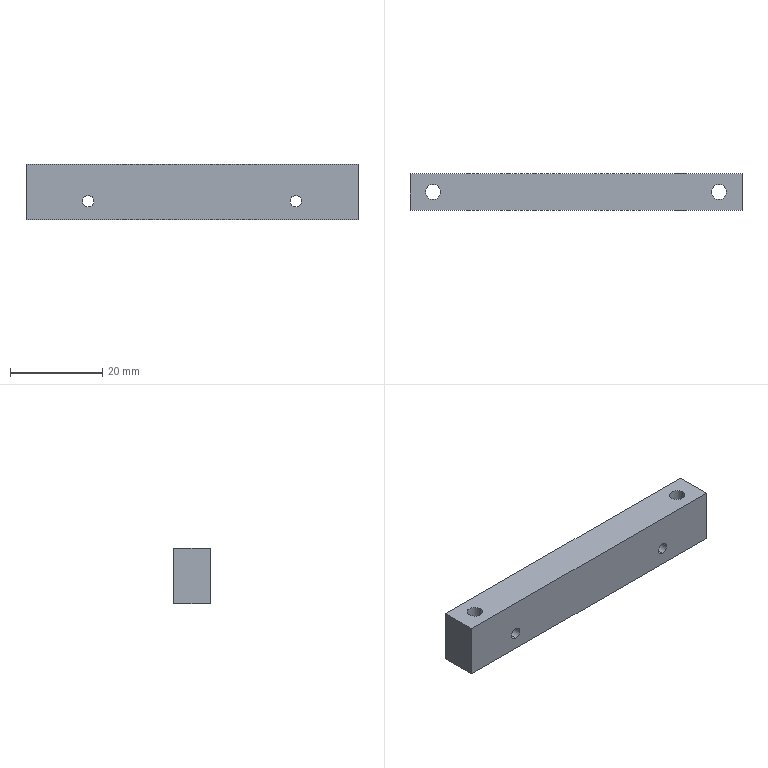Part | SolidWorks | features BaseBody 1 | 1 solid | 14 faces | box 72 x 8 x 12 mm | volume 6628 mm3 | cylinder 8 | plane 6 | commonest cylinder face diameters 2.5 x4 3.3 x4
STEP:
#1=CARTESIAN_POINT('',(22.5,-4.,2.75));
#2=VERTEX_POINT('',#1);
#3=CARTESIAN_POINT('',(22.5,-4.,5.25));
#4=VERTEX_POINT('',#3);
#5=CARTESIAN_POINT('',(22.5,-4.,4.));
#6=DIRECTION('',(0.,1.,0.));
#7=DIRECTION('',(0.,0.,1.));
#8=AXIS2_PLACEMENT_3D('',#5,#6,#7);
#9=CIRCLE('',#8,1.25);
#10=EDGE_CURVE('',#2,#4,#9,.T.);
#11=ORIENTED_EDGE('',*,*,#10,.F.);
#12=CARTESIAN_POINT('',(22.5,4.,2.75));
#13=VERTEX_POINT('',#12);
#14=CARTESIAN_POINT('',(22.5,4.,2.75));
#15=DIRECTION('',(0.,1.,0.));
#16=VECTOR('',#15,1000.);
#17=LINE('',#14,#16);
#18=EDGE_CURVE('',#2,#13,#17,.T.);
#19=ORIENTED_EDGE('',*,*,#18,.T.);
#20=CARTESIAN_POINT('',(22.5,4.,5.25));
#21=VERTEX_POINT('',#20);
#22=CARTESIAN_POINT('',(22.5,4.,4.));
#23=DIRECTION('',(0.,1.,0.));
#24=DIRECTION('',(0.,0.,1.));
#25=AXIS2_PLACEMENT_3D('',#22,#23,#24);
#26=CIRCLE('',#25,1.25);
#27=EDGE_CURVE('',#13,#21,#26,.T.);
#28=ORIENTED_EDGE('',*,*,#27,.T.);
#29=CARTESIAN_POINT('',(22.5,4.,5.25));
#30=DIRECTION('',(0.,1.,0.));
#31=VECTOR('',#30,1000.);
#32=LINE('',#29,#31);
#33=EDGE_CURVE('',#4,#21,#32,.T.);
#34=ORIENTED_EDGE('',*,*,#33,.F.);
#35=EDGE_LOOP('',(#11,#19,#28,#34));
#36=FACE_OUTER_BOUND('',#35,.T.);
#37=CARTESIAN_POINT('',(22.5,4.,4.));
#38=DIRECTION('',(0.,1.,0.));
#39=DIRECTION('',(0.,0.,1.));
#40=AXIS2_PLACEMENT_3D('',#37,#38,#39);
#41=CYLINDRICAL_SURFACE('',#40,1.25);
#42=ADVANCED_FACE('',(#36),#41,.F.);
#43=CARTESIAN_POINT('',(-22.5,-4.,2.75));
#44=VERTEX_POINT('',#43);
#45=CARTESIAN_POINT('',(-22.5,-4.,5.25));
#46=VERTEX_POINT('',#45);
#47=CARTESIAN_POINT('',(-22.5,-4.,4.));
#48=DIRECTION('',(0.,1.,0.));
#49=DIRECTION('',(0.,0.,1.));
#50=AXIS2_PLACEMENT_3D('',#47,#48,#49);
#51=CIRCLE('',#50,1.25);
#52=EDGE_CURVE('',#44,#46,#51,.T.);
#53=ORIENTED_EDGE('',*,*,#52,.F.);
#54=CARTESIAN_POINT('',(-22.5,4.,2.75));
#55=VERTEX_POINT('',#54);
#56=CARTESIAN_POINT('',(-22.5,4.,2.75));
#57=DIRECTION('',(0.,1.,0.));
#58=VECTOR('',#57,1000.);
#59=LINE('',#56,#58);
#60=EDGE_CURVE('',#44,#55,#59,.T.);
#61=ORIENTED_EDGE('',*,*,#60,.T.);
#62=CARTESIAN_POINT('',(-22.5,4.,5.25));
#63=VERTEX_POINT('',#62);
#64=CARTESIAN_POINT('',(-22.5,4.,4.));
#65=DIRECTION('',(0.,1.,0.));
#66=DIRECTION('',(0.,0.,1.));
#67=AXIS2_PLACEMENT_3D('',#64,#65,#66);
#68=CIRCLE('',#67,1.25);
#69=EDGE_CURVE('',#55,#63,#68,.T.);
#70=ORIENTED_EDGE('',*,*,#69,.T.);
#71=CARTESIAN_POINT('',(-22.5,4.,5.25));
#72=DIRECTION('',(0.,1.,0.));
#73=VECTOR('',#72,1000.);
#74=LINE('',#71,#73);
#75=EDGE_CURVE('',#46,#63,#74,.T.);
#76=ORIENTED_EDGE('',*,*,#75,.F.);
#77=EDGE_LOOP('',(#53,#61,#70,#76));
#78=FACE_OUTER_BOUND('',#77,.T.);
#79=CARTESIAN_POINT('',(-22.5,4.,4.));
#80=DIRECTION('',(0.,1.,0.));
#81=DIRECTION('',(0.,0.,1.));
#82=AXIS2_PLACEMENT_3D('',#79,#80,#81);
#83=CYLINDRICAL_SURFACE('',#82,1.25);
#84=ADVANCED_FACE('',(#78),#83,.F.);
#85=CARTESIAN_POINT('',(-32.65,0.,0.));
#86=VERTEX_POINT('',#85);
#87=CARTESIAN_POINT('',(-29.35,0.,0.));
#88=VERTEX_POINT('',#87);
#89=CARTESIAN_POINT('',(-31.,0.,0.));
#90=DIRECTION('',(0.,0.,1.));
#91=DIRECTION('',(1.,0.,0.));
#92=AXIS2_PLACEMENT_3D('',#89,#90,#91);
#93=CIRCLE('',#92,1.65);
#94=EDGE_CURVE('',#86,#88,#93,.T.);
#95=ORIENTED_EDGE('',*,*,#94,.F.);
#96=CARTESIAN_POINT('',(-32.65,0.,12.));
#97=VERTEX_POINT('',#96);
#98=CARTESIAN_POINT('',(-32.65,0.,12.));
#99=DIRECTION('',(0.,0.,1.));
#100=VECTOR('',#99,1000.);
#101=LINE('',#98,#100);
#102=EDGE_CURVE('',#86,#97,#101,.T.);
#103=ORIENTED_EDGE('',*,*,#102,.T.);
#104=CARTESIAN_POINT('',(-29.35,0.,12.));
#105=VERTEX_POINT('',#104);
#106=CARTESIAN_POINT('',(-31.,0.,12.));
#107=DIRECTION('',(0.,0.,1.));
#108=DIRECTION('',(1.,0.,0.));
#109=AXIS2_PLACEMENT_3D('',#106,#107,#108);
#110=CIRCLE('',#109,1.65);
#111=EDGE_CURVE('',#97,#105,#110,.T.);
#112=ORIENTED_EDGE('',*,*,#111,.T.);
#113=CARTESIAN_POINT('',(-29.35,0.,12.));
#114=DIRECTION('',(0.,0.,1.));
#115=VECTOR('',#114,1000.);
#116=LINE('',#113,#115);
#117=EDGE_CURVE('',#88,#105,#116,.T.);
#118=ORIENTED_EDGE('',*,*,#117,.F.);
#119=EDGE_LOOP('',(#95,#103,#112,#118));
#120=FACE_OUTER_BOUND('',#119,.T.);
#121=CARTESIAN_POINT('',(-31.,0.,12.));
#122=DIRECTION('',(0.,0.,1.));
#123=DIRECTION('',(1.,0.,0.));
#124=AXIS2_PLACEMENT_3D('',#121,#122,#123);
#125=CYLINDRICAL_SURFACE('',#124,1.65);
#126=ADVANCED_FACE('',(#120),#125,.F.);
#127=CARTESIAN_POINT('',(29.35,0.,0.));
#128=VERTEX_POINT('',#127);
#129=CARTESIAN_POINT('',(32.65,0.,0.));
#130=VERTEX_POINT('',#129);
#131=CARTESIAN_POINT('',(31.,0.,0.));
#132=DIRECTION('',(0.,0.,1.));
#133=DIRECTION('',(1.,0.,0.));
#134=AXIS2_PLACEMENT_3D('',#131,#132,#133);
#135=CIRCLE('',#134,1.65);
#136=EDGE_CURVE('',#128,#130,#135,.T.);
#137=ORIENTED_EDGE('',*,*,#136,.F.);
#138=CARTESIAN_POINT('',(29.35,0.,12.));
#139=VERTEX_POINT('',#138);
#140=CARTESIAN_POINT('',(29.35,0.,12.));
#141=DIRECTION('',(0.,0.,1.));
#142=VECTOR('',#141,1000.);
#143=LINE('',#140,#142);
#144=EDGE_CURVE('',#128,#139,#143,.T.);
#145=ORIENTED_EDGE('',*,*,#144,.T.);
#146=CARTESIAN_POINT('',(32.65,0.,12.));
#147=VERTEX_POINT('',#146);
#148=CARTESIAN_POINT('',(31.,0.,12.));
#149=DIRECTION('',(0.,0.,1.));
#150=DIRECTION('',(1.,0.,0.));
#151=AXIS2_PLACEMENT_3D('',#148,#149,#150);
#152=CIRCLE('',#151,1.65);
#153=EDGE_CURVE('',#139,#147,#152,.T.);
#154=ORIENTED_EDGE('',*,*,#153,.T.);
#155=CARTESIAN_POINT('',(32.65,0.,12.));
#156=DIRECTION('',(0.,0.,1.));
#157=VECTOR('',#156,1000.);
#158=LINE('',#155,#157);
#159=EDGE_CURVE('',#130,#147,#158,.T.);
#160=ORIENTED_EDGE('',*,*,#159,.F.);
#161=EDGE_LOOP('',(#137,#145,#154,#160));
#162=FACE_OUTER_BOUND('',#161,.T.);
#163=CARTESIAN_POINT('',(31.,0.,12.));
#164=DIRECTION('',(0.,0.,1.));
#165=DIRECTION('',(1.,0.,0.));
#166=AXIS2_PLACEMENT_3D('',#163,#164,#165);
#167=CYLINDRICAL_SURFACE('',#166,1.65);
#168=ADVANCED_FACE('',(#162),#167,.F.);
#169=CARTESIAN_POINT('',(-36.,4.,12.));
#170=VERTEX_POINT('',#169);
#171=CARTESIAN_POINT('',(-36.,4.,0.));
#172=VERTEX_POINT('',#171);
#173=CARTESIAN_POINT('',(-36.,4.,12.));
#174=DIRECTION('',(0.,0.,-1.));
#175=VECTOR('',#174,1000.);
#176=LINE('',#173,#175);
#177=EDGE_CURVE('',#170,#172,#176,.T.);
#178=ORIENTED_EDGE('',*,*,#177,.F.);
#179=CARTESIAN_POINT('',(36.,4.,12.));
#180=VERTEX_POINT('',#179);
#181=CARTESIAN_POINT('',(-36.,4.,12.));
#182=DIRECTION('',(-1.,0.,0.));
#183=VECTOR('',#182,1000.);
#184=LINE('',#181,#183);
#185=EDGE_CURVE('',#180,#170,#184,.T.);
#186=ORIENTED_EDGE('',*,*,#185,.F.);
#187=CARTESIAN_POINT('',(36.,4.,0.));
#188=VERTEX_POINT('',#187);
#189=CARTESIAN_POINT('',(36.,4.,12.));
#190=DIRECTION('',(0.,0.,1.));
#191=VECTOR('',#190,1000.);
#192=LINE('',#189,#191);
#193=EDGE_CURVE('',#188,#180,#192,.T.);
#194=ORIENTED_EDGE('',*,*,#193,.F.);
#195=CARTESIAN_POINT('',(-36.,4.,0.));
#196=DIRECTION('',(1.,0.,0.));
#197=VECTOR('',#196,1000.);
#198=LINE('',#195,#197);
#199=EDGE_CURVE('',#172,#188,#198,.T.);
#200=ORIENTED_EDGE('',*,*,#199,.F.);
#201=EDGE_LOOP('',(#178,#186,#194,#200));
#202=FACE_OUTER_BOUND('',#201,.T.);
#203=CARTESIAN_POINT('',(22.5,4.,4.));
#204=DIRECTION('',(0.,1.,0.));
#205=DIRECTION('',(0.,0.,1.));
#206=AXIS2_PLACEMENT_3D('',#203,#204,#205);
#207=CIRCLE('',#206,1.25);
#208=EDGE_CURVE('',#21,#13,#207,.T.);
#209=ORIENTED_EDGE('',*,*,#208,.F.);
#210=ORIENTED_EDGE('',*,*,#27,.F.);
#211=EDGE_LOOP('',(#209,#210));
#212=FACE_BOUND('',#211,.T.);
#213=CARTESIAN_POINT('',(-22.5,4.,4.));
#214=DIRECTION('',(0.,1.,0.));
#215=DIRECTION('',(0.,0.,1.));
#216=AXIS2_PLACEMENT_3D('',#213,#214,#215);
#217=CIRCLE('',#216,1.25);
#218=EDGE_CURVE('',#63,#55,#217,.T.);
#219=ORIENTED_EDGE('',*,*,#218,.F.);
#220=ORIENTED_EDGE('',*,*,#69,.F.);
#221=EDGE_LOOP('',(#219,#220));
#222=FACE_BOUND('',#221,.T.);
#223=CARTESIAN_POINT('',(-36.,4.,12.));
#224=DIRECTION('',(0.,-1.,0.));
#225=DIRECTION('',(0.,0.,-1.));
#226=AXIS2_PLACEMENT_3D('',#223,#224,#225);
#227=PLANE('',#226);
#228=ADVANCED_FACE('',(#202,#212,#222),#227,.F.);
#229=CARTESIAN_POINT('',(-36.,-4.,0.));
#230=VERTEX_POINT('',#229);
#231=CARTESIAN_POINT('',(-36.,0.,0.));
#232=DIRECTION('',(0.,1.,0.));
#233=VECTOR('',#232,1000.);
#234=LINE('',#231,#233);
#235=EDGE_CURVE('',#230,#172,#234,.T.);
#236=ORIENTED_EDGE('',*,*,#235,.T.);
#237=ORIENTED_EDGE('',*,*,#199,.T.);
#238=CARTESIAN_POINT('',(36.,-4.,0.));
#239=VERTEX_POINT('',#238);
#240=CARTESIAN_POINT('',(36.,0.,0.));
#241=DIRECTION('',(0.,-1.,0.));
#242=VECTOR('',#241,1000.);
#243=LINE('',#240,#242);
#244=EDGE_CURVE('',#188,#239,#243,.T.);
#245=ORIENTED_EDGE('',*,*,#244,.T.);
#246=CARTESIAN_POINT('',(0.,-4.,0.));
#247=DIRECTION('',(-1.,0.,0.));
#248=VECTOR('',#247,1000.);
#249=LINE('',#246,#248);
#250=EDGE_CURVE('',#239,#230,#249,.T.);
#251=ORIENTED_EDGE('',*,*,#250,.T.);
#252=EDGE_LOOP('',(#236,#237,#245,#251));
#253=FACE_OUTER_BOUND('',#252,.T.);
#254=CARTESIAN_POINT('',(-31.,0.,0.));
#255=DIRECTION('',(0.,0.,1.));
#256=DIRECTION('',(1.,0.,0.));
#257=AXIS2_PLACEMENT_3D('',#254,#255,#256);
#258=CIRCLE('',#257,1.65);
#259=EDGE_CURVE('',#88,#86,#258,.T.);
#260=ORIENTED_EDGE('',*,*,#259,.T.);
#261=ORIENTED_EDGE('',*,*,#94,.T.);
#262=EDGE_LOOP('',(#260,#261));
#263=FACE_BOUND('',#262,.T.);
#264=CARTESIAN_POINT('',(31.,0.,0.));
#265=DIRECTION('',(0.,0.,1.));
#266=DIRECTION('',(1.,0.,0.));
#267=AXIS2_PLACEMENT_3D('',#264,#265,#266);
#268=CIRCLE('',#267,1.65);
#269=EDGE_CURVE('',#130,#128,#268,.T.);
#270=ORIENTED_EDGE('',*,*,#269,.T.);
#271=ORIENTED_EDGE('',*,*,#136,.T.);
#272=EDGE_LOOP('',(#270,#271));
#273=FACE_BOUND('',#272,.T.);
#274=CARTESIAN_POINT('',(0.,0.,0.));
#275=DIRECTION('',(0.,0.,-1.));
#276=DIRECTION('',(-1.,0.,0.));
#277=AXIS2_PLACEMENT_3D('',#274,#275,#276);
#278=PLANE('',#277);
#279=ADVANCED_FACE('',(#253,#263,#273),#278,.T.);
#280=CARTESIAN_POINT('',(-36.,-4.,12.));
#281=VERTEX_POINT('',#280);
#282=CARTESIAN_POINT('',(-36.,-4.,12.));
#283=DIRECTION('',(0.,0.,-1.));
#284=VECTOR('',#283,1000.);
#285=LINE('',#282,#284);
#286=EDGE_CURVE('',#281,#230,#285,.T.);
#287=ORIENTED_EDGE('',*,*,#286,.F.);
#288=CARTESIAN_POINT('',(-36.,-4.,12.));
#289=DIRECTION('',(0.,-1.,0.));
#290=VECTOR('',#289,1000.);
#291=LINE('',#288,#290);
#292=EDGE_CURVE('',#170,#281,#291,.T.);
#293=ORIENTED_EDGE('',*,*,#292,.F.);
#294=ORIENTED_EDGE('',*,*,#177,.T.);
#295=ORIENTED_EDGE('',*,*,#235,.F.);
#296=EDGE_LOOP('',(#287,#293,#294,#295));
#297=FACE_OUTER_BOUND('',#296,.T.);
#298=CARTESIAN_POINT('',(-36.,-4.,12.));
#299=DIRECTION('',(1.,0.,0.));
#300=DIRECTION('',(0.,0.,-1.));
#301=AXIS2_PLACEMENT_3D('',#298,#299,#300);
#302=PLANE('',#301);
#303=ADVANCED_FACE('',(#297),#302,.F.);
#304=ORIENTED_EDGE('',*,*,#185,.T.);
#305=ORIENTED_EDGE('',*,*,#292,.T.);
#306=CARTESIAN_POINT('',(36.,-4.,12.));
#307=VERTEX_POINT('',#306);
#308=CARTESIAN_POINT('',(0.,-4.,12.));
#309=DIRECTION('',(-1.,0.,0.));
#310=VECTOR('',#309,1000.);
#311=LINE('',#308,#310);
#312=EDGE_CURVE('',#307,#281,#311,.T.);
#313=ORIENTED_EDGE('',*,*,#312,.F.);
#314=CARTESIAN_POINT('',(36.,0.,12.));
#315=DIRECTION('',(0.,-1.,0.));
#316=VECTOR('',#315,1000.);
#317=LINE('',#314,#316);
#318=EDGE_CURVE('',#180,#307,#317,.T.);
#319=ORIENTED_EDGE('',*,*,#318,.F.);
#320=EDGE_LOOP('',(#304,#305,#313,#319));
#321=FACE_OUTER_BOUND('',#320,.T.);
#322=CARTESIAN_POINT('',(-31.,0.,12.));
#323=DIRECTION('',(0.,0.,1.));
#324=DIRECTION('',(1.,0.,0.));
#325=AXIS2_PLACEMENT_3D('',#322,#323,#324);
#326=CIRCLE('',#325,1.65);
#327=EDGE_CURVE('',#105,#97,#326,.T.);
#328=ORIENTED_EDGE('',*,*,#327,.F.);
#329=ORIENTED_EDGE('',*,*,#111,.F.);
#330=EDGE_LOOP('',(#328,#329));
#331=FACE_BOUND('',#330,.T.);
#332=CARTESIAN_POINT('',(31.,0.,12.));
#333=DIRECTION('',(0.,0.,1.));
#334=DIRECTION('',(1.,0.,0.));
#335=AXIS2_PLACEMENT_3D('',#332,#333,#334);
#336=CIRCLE('',#335,1.65);
#337=EDGE_CURVE('',#147,#139,#336,.T.);
#338=ORIENTED_EDGE('',*,*,#337,.F.);
#339=ORIENTED_EDGE('',*,*,#153,.F.);
#340=EDGE_LOOP('',(#338,#339));
#341=FACE_BOUND('',#340,.T.);
#342=CARTESIAN_POINT('',(0.,0.,12.));
#343=DIRECTION('',(0.,0.,-1.));
#344=DIRECTION('',(-1.,0.,0.));
#345=AXIS2_PLACEMENT_3D('',#342,#343,#344);
#346=PLANE('',#345);
#347=ADVANCED_FACE('',(#321,#331,#341),#346,.F.);
#348=ORIENTED_EDGE('',*,*,#193,.T.);
#349=ORIENTED_EDGE('',*,*,#318,.T.);
#350=CARTESIAN_POINT('',(36.,-4.,12.));
#351=DIRECTION('',(0.,0.,1.));
#352=VECTOR('',#351,1000.);
#353=LINE('',#350,#352);
#354=EDGE_CURVE('',#239,#307,#353,.T.);
#355=ORIENTED_EDGE('',*,*,#354,.F.);
#356=ORIENTED_EDGE('',*,*,#244,.F.);
#357=EDGE_LOOP('',(#348,#349,#355,#356));
#358=FACE_OUTER_BOUND('',#357,.T.);
#359=CARTESIAN_POINT('',(36.,-4.,12.));
#360=DIRECTION('',(-1.,0.,0.));
#361=DIRECTION('',(0.,0.,1.));
#362=AXIS2_PLACEMENT_3D('',#359,#360,#361);
#363=PLANE('',#362);
#364=ADVANCED_FACE('',(#358),#363,.F.);
#365=ORIENTED_EDGE('',*,*,#18,.F.);
#366=CARTESIAN_POINT('',(22.5,-4.,4.));
#367=DIRECTION('',(0.,1.,0.));
#368=DIRECTION('',(0.,0.,1.));
#369=AXIS2_PLACEMENT_3D('',#366,#367,#368);
#370=CIRCLE('',#369,1.25);
#371=EDGE_CURVE('',#4,#2,#370,.T.);
#372=ORIENTED_EDGE('',*,*,#371,.F.);
#373=ORIENTED_EDGE('',*,*,#33,.T.);
#374=ORIENTED_EDGE('',*,*,#208,.T.);
#375=EDGE_LOOP('',(#365,#372,#373,#374));
#376=FACE_OUTER_BOUND('',#375,.T.);
#377=CARTESIAN_POINT('',(22.5,4.,4.));
#378=DIRECTION('',(0.,1.,0.));
#379=DIRECTION('',(0.,0.,1.));
#380=AXIS2_PLACEMENT_3D('',#377,#378,#379);
#381=CYLINDRICAL_SURFACE('',#380,1.25);
#382=ADVANCED_FACE('',(#376),#381,.F.);
#383=ORIENTED_EDGE('',*,*,#60,.F.);
#384=CARTESIAN_POINT('',(-22.5,-4.,4.));
#385=DIRECTION('',(0.,1.,0.));
#386=DIRECTION('',(0.,0.,1.));
#387=AXIS2_PLACEMENT_3D('',#384,#385,#386);
#388=CIRCLE('',#387,1.25);
#389=EDGE_CURVE('',#46,#44,#388,.T.);
#390=ORIENTED_EDGE('',*,*,#389,.F.);
#391=ORIENTED_EDGE('',*,*,#75,.T.);
#392=ORIENTED_EDGE('',*,*,#218,.T.);
#393=EDGE_LOOP('',(#383,#390,#391,#392));
#394=FACE_OUTER_BOUND('',#393,.T.);
#395=CARTESIAN_POINT('',(-22.5,4.,4.));
#396=DIRECTION('',(0.,1.,0.));
#397=DIRECTION('',(0.,0.,1.));
#398=AXIS2_PLACEMENT_3D('',#395,#396,#397);
#399=CYLINDRICAL_SURFACE('',#398,1.25);
#400=ADVANCED_FACE('',(#394),#399,.F.);
#401=ORIENTED_EDGE('',*,*,#354,.T.);
#402=ORIENTED_EDGE('',*,*,#312,.T.);
#403=ORIENTED_EDGE('',*,*,#286,.T.);
#404=ORIENTED_EDGE('',*,*,#250,.F.);
#405=EDGE_LOOP('',(#401,#402,#403,#404));
#406=FACE_OUTER_BOUND('',#405,.T.);
#407=ORIENTED_EDGE('',*,*,#371,.T.);
#408=ORIENTED_EDGE('',*,*,#10,.T.);
#409=EDGE_LOOP('',(#407,#408));
#410=FACE_BOUND('',#409,.T.);
#411=ORIENTED_EDGE('',*,*,#389,.T.);
#412=ORIENTED_EDGE('',*,*,#52,.T.);
#413=EDGE_LOOP('',(#411,#412));
#414=FACE_BOUND('',#413,.T.);
#415=CARTESIAN_POINT('',(-36.,-4.,12.));
#416=DIRECTION('',(0.,1.,0.));
#417=DIRECTION('',(0.,0.,1.));
#418=AXIS2_PLACEMENT_3D('',#415,#416,#417);
#419=PLANE('',#418);
#420=ADVANCED_FACE('',(#406,#410,#414),#419,.F.);
#421=ORIENTED_EDGE('',*,*,#102,.F.);
#422=ORIENTED_EDGE('',*,*,#259,.F.);
#423=ORIENTED_EDGE('',*,*,#117,.T.);
#424=ORIENTED_EDGE('',*,*,#327,.T.);
#425=EDGE_LOOP('',(#421,#422,#423,#424));
#426=FACE_OUTER_BOUND('',#425,.T.);
#427=CARTESIAN_POINT('',(-31.,0.,12.));
#428=DIRECTION('',(0.,0.,1.));
#429=DIRECTION('',(1.,0.,0.));
#430=AXIS2_PLACEMENT_3D('',#427,#428,#429);
#431=CYLINDRICAL_SURFACE('',#430,1.65);
#432=ADVANCED_FACE('',(#426),#431,.F.);
#433=ORIENTED_EDGE('',*,*,#144,.F.);
#434=ORIENTED_EDGE('',*,*,#269,.F.);
#435=ORIENTED_EDGE('',*,*,#159,.T.);
#436=ORIENTED_EDGE('',*,*,#337,.T.);
#437=EDGE_LOOP('',(#433,#434,#435,#436));
#438=FACE_OUTER_BOUND('',#437,.T.);
#439=CARTESIAN_POINT('',(31.,0.,12.));
#440=DIRECTION('',(0.,0.,1.));
#441=DIRECTION('',(1.,0.,0.));
#442=AXIS2_PLACEMENT_3D('',#439,#440,#441);
#443=CYLINDRICAL_SURFACE('',#442,1.65);
#444=ADVANCED_FACE('',(#438),#443,.F.);
#445=CLOSED_SHELL('',(#42,#84,#126,#168,#228,#279,#303,#347,#364,#382,#400,#420,#432,#444));
#446=MANIFOLD_SOLID_BREP('',#445);
#447=CARTESIAN_POINT('',(0.,0.,0.));
#448=DIRECTION('',(0.,0.,1.));
#449=DIRECTION('',(1.,0.,0.));
#450=AXIS2_PLACEMENT_3D('',#447,#448,#449);
#451=(LENGTH_UNIT()NAMED_UNIT(*)SI_UNIT(.MILLI.,.METRE.));
#452=UNCERTAINTY_MEASURE_WITH_UNIT(LENGTH_MEASURE(0.00001),#451,'','');
#453=(NAMED_UNIT(*)PLANE_ANGLE_UNIT()SI_UNIT($,.RADIAN.));
#454=(NAMED_UNIT(*)SI_UNIT($,.STERADIAN.)SOLID_ANGLE_UNIT());
#455=(GEOMETRIC_REPRESENTATION_CONTEXT(3)GLOBAL_UNCERTAINTY_ASSIGNED_CONTEXT((#452))GLOBAL_UNIT_ASSIGNED_CONTEXT((#451,#453,#454))REPRESENTATION_CONTEXT('',''));
#456=ADVANCED_BREP_SHAPE_REPRESENTATION('',(#446,#450),#455);